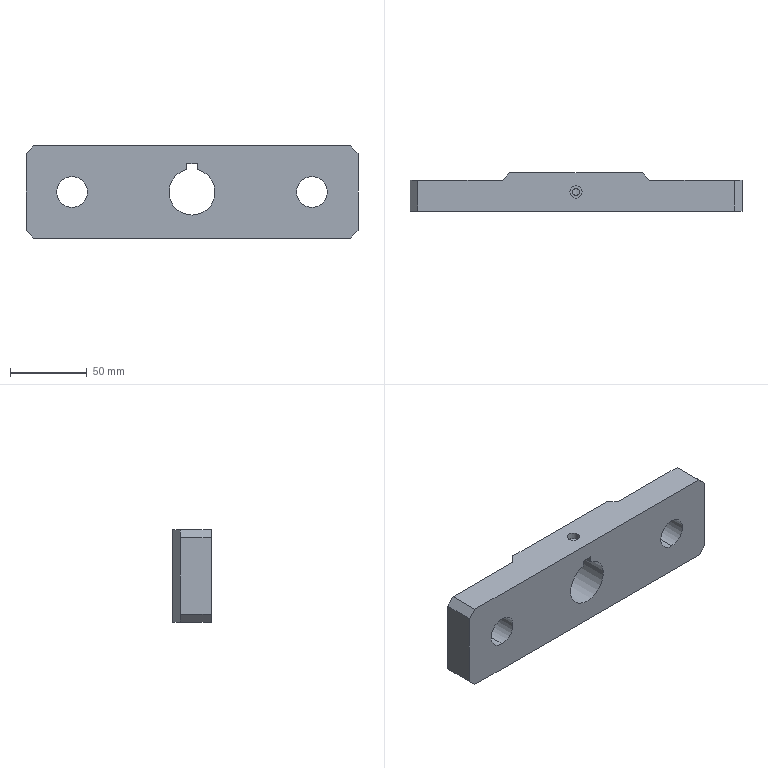Part | STEP file | BU-A12 | 1 solid | 63 faces | box 216 x 25 x 60 mm | volume 252234 mm3 | cylinder 27 | cone 18 | plane 18 | commonest cylinder face diameters 5 x16 20 x4 3.3 x2 4.5 x2 8 x2 30 x1